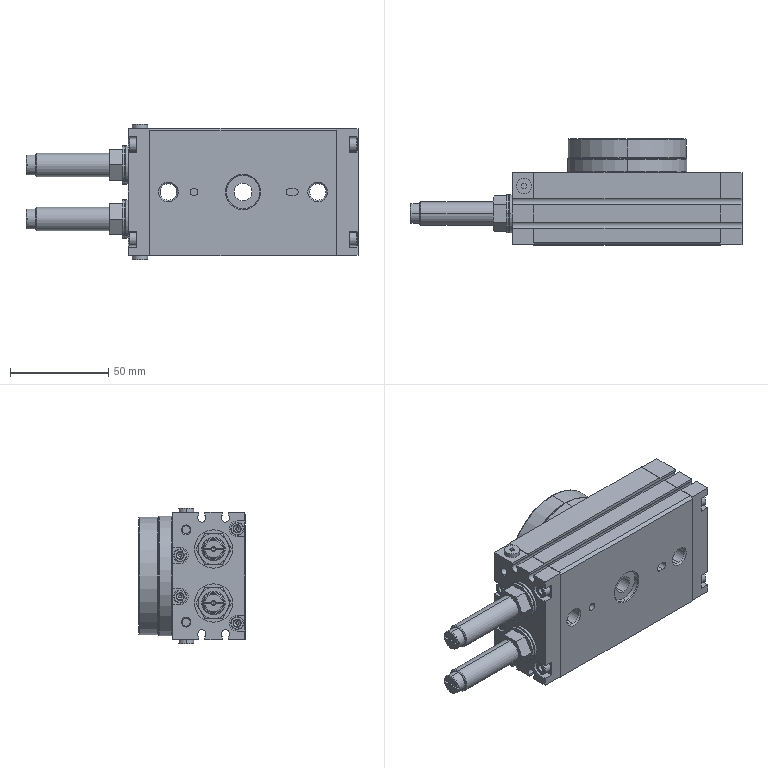Part | SolidWorks | features BaseBody 1 | 1 solid | 530 faces | box 169 x 54 x 69 mm | volume 316478 mm3 | plane 188 | cylinder 170 | cone 144 | torus 28 | commonest cylinder face diameters 6.66 x28 4.917 x24 3.5 x16 2.572 x12 4 x12 6.16 x12